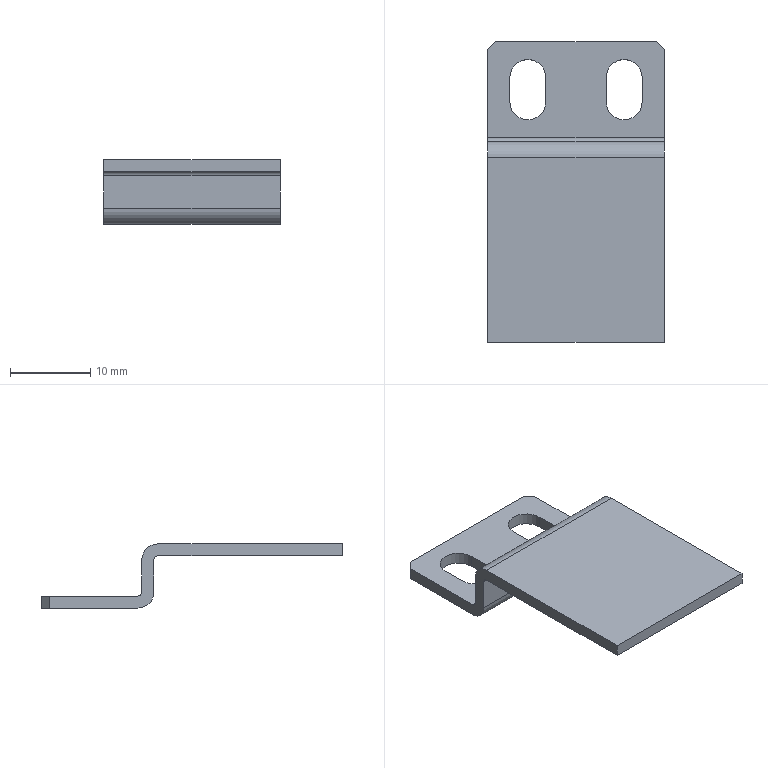Part | SolidWorks | features BaseBody 1 | 1 solid | 24 faces | box 22 x 37.5 x 8 mm | volume 1327 mm3 | plane 16 | cylinder 8 | commonest cylinder face diameters 4.5 x4 1 x2 4 x2
STEP:
#1=CARTESIAN_POINT('',(0.,-37.5,6.5));
#2=VERTEX_POINT('',#1);
#3=CARTESIAN_POINT('',(0.,-14.5,6.5));
#4=VERTEX_POINT('',#3);
#5=CARTESIAN_POINT('',(0.,0.,6.5));
#6=DIRECTION('',(0.,1.,0.));
#7=VECTOR('',#6,1000.);
#8=LINE('',#5,#7);
#9=EDGE_CURVE('',#2,#4,#8,.T.);
#10=ORIENTED_EDGE('',*,*,#9,.F.);
#11=CARTESIAN_POINT('',(22.,-37.5,6.5));
#12=VERTEX_POINT('',#11);
#13=CARTESIAN_POINT('',(0.,-37.5,6.5));
#14=DIRECTION('',(-1.,0.,0.));
#15=VECTOR('',#14,1000.);
#16=LINE('',#13,#15);
#17=EDGE_CURVE('',#12,#2,#16,.T.);
#18=ORIENTED_EDGE('',*,*,#17,.F.);
#19=CARTESIAN_POINT('',(22.,-14.5,6.5));
#20=VERTEX_POINT('',#19);
#21=CARTESIAN_POINT('',(22.,0.,6.5));
#22=DIRECTION('',(0.,-1.,0.));
#23=VECTOR('',#22,1000.);
#24=LINE('',#21,#23);
#25=EDGE_CURVE('',#20,#12,#24,.T.);
#26=ORIENTED_EDGE('',*,*,#25,.F.);
#27=CARTESIAN_POINT('',(0.,-14.5,6.5));
#28=DIRECTION('',(1.,0.,0.));
#29=VECTOR('',#28,1000.);
#30=LINE('',#27,#29);
#31=EDGE_CURVE('',#4,#20,#30,.T.);
#32=ORIENTED_EDGE('',*,*,#31,.F.);
#33=EDGE_LOOP('',(#10,#18,#26,#32));
#34=FACE_OUTER_BOUND('',#33,.T.);
#35=CARTESIAN_POINT('',(0.,0.,6.5));
#36=DIRECTION('',(0.,0.,-1.));
#37=DIRECTION('',(0.,1.,0.));
#38=AXIS2_PLACEMENT_3D('',#35,#36,#37);
#39=PLANE('',#38);
#40=ADVANCED_FACE('',(#34),#39,.F.);
#41=ORIENTED_EDGE('',*,*,#31,.T.);
#42=CARTESIAN_POINT('',(22.,-12.5,4.5));
#43=VERTEX_POINT('',#42);
#44=CARTESIAN_POINT('',(22.,-14.5,4.5));
#45=DIRECTION('',(-1.,0.,0.));
#46=DIRECTION('',(0.,0.,1.));
#47=AXIS2_PLACEMENT_3D('',#44,#45,#46);
#48=CIRCLE('',#47,2.);
#49=EDGE_CURVE('',#20,#43,#48,.T.);
#50=ORIENTED_EDGE('',*,*,#49,.T.);
#51=CARTESIAN_POINT('',(0.,-12.5,4.5));
#52=VERTEX_POINT('',#51);
#53=CARTESIAN_POINT('',(0.,-12.5,4.5));
#54=DIRECTION('',(-1.,0.,0.));
#55=VECTOR('',#54,1000.);
#56=LINE('',#53,#55);
#57=EDGE_CURVE('',#43,#52,#56,.T.);
#58=ORIENTED_EDGE('',*,*,#57,.T.);
#59=CARTESIAN_POINT('',(0.,-14.5,4.5));
#60=DIRECTION('',(1.,0.,0.));
#61=DIRECTION('',(0.,0.,1.));
#62=AXIS2_PLACEMENT_3D('',#59,#60,#61);
#63=CIRCLE('',#62,2.);
#64=EDGE_CURVE('',#52,#4,#63,.T.);
#65=ORIENTED_EDGE('',*,*,#64,.T.);
#66=EDGE_LOOP('',(#41,#50,#58,#65));
#67=FACE_OUTER_BOUND('',#66,.T.);
#68=CARTESIAN_POINT('',(0.,-14.5,4.5));
#69=DIRECTION('',(-1.,0.,0.));
#70=DIRECTION('',(0.,0.,1.));
#71=AXIS2_PLACEMENT_3D('',#68,#69,#70);
#72=CYLINDRICAL_SURFACE('',#71,2.);
#73=ADVANCED_FACE('',(#67),#72,.T.);
#74=CARTESIAN_POINT('',(0.,-37.5,5.));
#75=VERTEX_POINT('',#74);
#76=CARTESIAN_POINT('',(0.,-14.5,5.));
#77=VERTEX_POINT('',#76);
#78=CARTESIAN_POINT('',(0.,-37.5,5.));
#79=DIRECTION('',(0.,1.,0.));
#80=VECTOR('',#79,1000.);
#81=LINE('',#78,#80);
#82=EDGE_CURVE('',#75,#77,#81,.T.);
#83=ORIENTED_EDGE('',*,*,#82,.F.);
#84=CARTESIAN_POINT('',(0.,-37.5,6.5));
#85=DIRECTION('',(0.,0.,-1.));
#86=VECTOR('',#85,1000.);
#87=LINE('',#84,#86);
#88=EDGE_CURVE('',#2,#75,#87,.T.);
#89=ORIENTED_EDGE('',*,*,#88,.F.);
#90=ORIENTED_EDGE('',*,*,#9,.T.);
#91=ORIENTED_EDGE('',*,*,#64,.F.);
#92=CARTESIAN_POINT('',(0.,-12.5,0.5));
#93=VERTEX_POINT('',#92);
#94=CARTESIAN_POINT('',(0.,-12.5,0.));
#95=DIRECTION('',(0.,0.,1.));
#96=VECTOR('',#95,1000.);
#97=LINE('',#94,#96);
#98=EDGE_CURVE('',#93,#52,#97,.T.);
#99=ORIENTED_EDGE('',*,*,#98,.F.);
#100=CARTESIAN_POINT('',(0.,-12.,0.));
#101=VERTEX_POINT('',#100);
#102=CARTESIAN_POINT('',(0.,-12.,0.5));
#103=DIRECTION('',(1.,0.,0.));
#104=DIRECTION('',(0.,0.,-1.));
#105=AXIS2_PLACEMENT_3D('',#102,#103,#104);
#106=CIRCLE('',#105,0.5);
#107=EDGE_CURVE('',#93,#101,#106,.T.);
#108=ORIENTED_EDGE('',*,*,#107,.T.);
#109=CARTESIAN_POINT('',(0.,-1.,0.));
#110=VERTEX_POINT('',#109);
#111=CARTESIAN_POINT('',(0.,0.,0.));
#112=DIRECTION('',(0.,-1.,0.));
#113=VECTOR('',#112,1000.);
#114=LINE('',#111,#113);
#115=EDGE_CURVE('',#110,#101,#114,.T.);
#116=ORIENTED_EDGE('',*,*,#115,.F.);
#117=CARTESIAN_POINT('',(0.,-1.,-1.5));
#118=VERTEX_POINT('',#117);
#119=CARTESIAN_POINT('',(0.,-1.,-1.5));
#120=DIRECTION('',(0.,0.,-1.));
#121=VECTOR('',#120,1000.);
#122=LINE('',#119,#121);
#123=EDGE_CURVE('',#110,#118,#122,.T.);
#124=ORIENTED_EDGE('',*,*,#123,.T.);
#125=CARTESIAN_POINT('',(0.,-12.,-1.5));
#126=VERTEX_POINT('',#125);
#127=CARTESIAN_POINT('',(0.,0.,-1.5));
#128=DIRECTION('',(0.,-1.,0.));
#129=VECTOR('',#128,1000.);
#130=LINE('',#127,#129);
#131=EDGE_CURVE('',#118,#126,#130,.T.);
#132=ORIENTED_EDGE('',*,*,#131,.T.);
#133=CARTESIAN_POINT('',(0.,-14.,0.5));
#134=VERTEX_POINT('',#133);
#135=CARTESIAN_POINT('',(0.,-12.,0.5));
#136=DIRECTION('',(1.,0.,0.));
#137=DIRECTION('',(0.,0.,-1.));
#138=AXIS2_PLACEMENT_3D('',#135,#136,#137);
#139=CIRCLE('',#138,2.);
#140=EDGE_CURVE('',#134,#126,#139,.T.);
#141=ORIENTED_EDGE('',*,*,#140,.F.);
#142=CARTESIAN_POINT('',(0.,-14.,4.5));
#143=VERTEX_POINT('',#142);
#144=CARTESIAN_POINT('',(0.,-14.,0.));
#145=DIRECTION('',(0.,0.,-1.));
#146=VECTOR('',#145,1000.);
#147=LINE('',#144,#146);
#148=EDGE_CURVE('',#143,#134,#147,.T.);
#149=ORIENTED_EDGE('',*,*,#148,.F.);
#150=CARTESIAN_POINT('',(0.,-14.5,4.5));
#151=DIRECTION('',(1.,0.,0.));
#152=DIRECTION('',(0.,0.,1.));
#153=AXIS2_PLACEMENT_3D('',#150,#151,#152);
#154=CIRCLE('',#153,0.5);
#155=EDGE_CURVE('',#143,#77,#154,.T.);
#156=ORIENTED_EDGE('',*,*,#155,.T.);
#157=EDGE_LOOP('',(#83,#89,#90,#91,#99,#108,#116,#124,#132,#141,#149,#156));
#158=FACE_OUTER_BOUND('',#157,.T.);
#159=CARTESIAN_POINT('',(0.,-37.5,6.5));
#160=DIRECTION('',(1.,0.,0.));
#161=DIRECTION('',(0.,0.,-1.));
#162=AXIS2_PLACEMENT_3D('',#159,#160,#161);
#163=PLANE('',#162);
#164=ADVANCED_FACE('',(#158),#163,.F.);
#165=CARTESIAN_POINT('',(22.,-37.5,5.));
#166=VERTEX_POINT('',#165);
#167=CARTESIAN_POINT('',(22.,-37.5,6.5));
#168=DIRECTION('',(0.,0.,-1.));
#169=VECTOR('',#168,1000.);
#170=LINE('',#167,#169);
#171=EDGE_CURVE('',#12,#166,#170,.T.);
#172=ORIENTED_EDGE('',*,*,#171,.F.);
#173=ORIENTED_EDGE('',*,*,#17,.T.);
#174=ORIENTED_EDGE('',*,*,#88,.T.);
#175=CARTESIAN_POINT('',(22.,-37.5,5.));
#176=DIRECTION('',(-1.,0.,0.));
#177=VECTOR('',#176,1000.);
#178=LINE('',#175,#177);
#179=EDGE_CURVE('',#166,#75,#178,.T.);
#180=ORIENTED_EDGE('',*,*,#179,.F.);
#181=EDGE_LOOP('',(#172,#173,#174,#180));
#182=FACE_OUTER_BOUND('',#181,.T.);
#183=CARTESIAN_POINT('',(22.,-37.5,6.5));
#184=DIRECTION('',(0.,1.,0.));
#185=DIRECTION('',(0.,0.,1.));
#186=AXIS2_PLACEMENT_3D('',#183,#184,#185);
#187=PLANE('',#186);
#188=ADVANCED_FACE('',(#182),#187,.F.);
#189=ORIENTED_EDGE('',*,*,#25,.T.);
#190=ORIENTED_EDGE('',*,*,#171,.T.);
#191=CARTESIAN_POINT('',(22.,-14.5,5.));
#192=VERTEX_POINT('',#191);
#193=CARTESIAN_POINT('',(22.,-14.,5.));
#194=DIRECTION('',(0.,-1.,0.));
#195=VECTOR('',#194,1000.);
#196=LINE('',#193,#195);
#197=EDGE_CURVE('',#192,#166,#196,.T.);
#198=ORIENTED_EDGE('',*,*,#197,.F.);
#199=CARTESIAN_POINT('',(22.,-14.,4.5));
#200=VERTEX_POINT('',#199);
#201=CARTESIAN_POINT('',(22.,-14.5,4.5));
#202=DIRECTION('',(-1.,0.,0.));
#203=DIRECTION('',(0.,0.,1.));
#204=AXIS2_PLACEMENT_3D('',#201,#202,#203);
#205=CIRCLE('',#204,0.5);
#206=EDGE_CURVE('',#192,#200,#205,.T.);
#207=ORIENTED_EDGE('',*,*,#206,.T.);
#208=CARTESIAN_POINT('',(22.,-14.,0.5));
#209=VERTEX_POINT('',#208);
#210=CARTESIAN_POINT('',(22.,-14.,4.5));
#211=DIRECTION('',(0.,0.,1.));
#212=VECTOR('',#211,1000.);
#213=LINE('',#210,#212);
#214=EDGE_CURVE('',#209,#200,#213,.T.);
#215=ORIENTED_EDGE('',*,*,#214,.F.);
#216=CARTESIAN_POINT('',(22.,-12.,-1.5));
#217=VERTEX_POINT('',#216);
#218=CARTESIAN_POINT('',(22.,-12.,0.5));
#219=DIRECTION('',(-1.,0.,0.));
#220=DIRECTION('',(0.,0.,-1.));
#221=AXIS2_PLACEMENT_3D('',#218,#219,#220);
#222=CIRCLE('',#221,2.);
#223=EDGE_CURVE('',#217,#209,#222,.T.);
#224=ORIENTED_EDGE('',*,*,#223,.F.);
#225=CARTESIAN_POINT('',(22.,-1.,-1.5));
#226=VERTEX_POINT('',#225);
#227=CARTESIAN_POINT('',(22.,0.,-1.5));
#228=DIRECTION('',(0.,1.,0.));
#229=VECTOR('',#228,1000.);
#230=LINE('',#227,#229);
#231=EDGE_CURVE('',#217,#226,#230,.T.);
#232=ORIENTED_EDGE('',*,*,#231,.T.);
#233=CARTESIAN_POINT('',(22.,-1.,0.));
#234=VERTEX_POINT('',#233);
#235=CARTESIAN_POINT('',(22.,-1.,-1.5));
#236=DIRECTION('',(0.,0.,1.));
#237=VECTOR('',#236,1000.);
#238=LINE('',#235,#237);
#239=EDGE_CURVE('',#226,#234,#238,.T.);
#240=ORIENTED_EDGE('',*,*,#239,.T.);
#241=CARTESIAN_POINT('',(22.,-12.,0.));
#242=VERTEX_POINT('',#241);
#243=CARTESIAN_POINT('',(22.,0.,0.));
#244=DIRECTION('',(0.,1.,0.));
#245=VECTOR('',#244,1000.);
#246=LINE('',#243,#245);
#247=EDGE_CURVE('',#242,#234,#246,.T.);
#248=ORIENTED_EDGE('',*,*,#247,.F.);
#249=CARTESIAN_POINT('',(22.,-12.5,0.5));
#250=VERTEX_POINT('',#249);
#251=CARTESIAN_POINT('',(22.,-12.,0.5));
#252=DIRECTION('',(1.,0.,0.));
#253=DIRECTION('',(0.,0.,-1.));
#254=AXIS2_PLACEMENT_3D('',#251,#252,#253);
#255=CIRCLE('',#254,0.5);
#256=EDGE_CURVE('',#250,#242,#255,.T.);
#257=ORIENTED_EDGE('',*,*,#256,.F.);
#258=CARTESIAN_POINT('',(22.,-12.5,0.));
#259=DIRECTION('',(0.,0.,-1.));
#260=VECTOR('',#259,1000.);
#261=LINE('',#258,#260);
#262=EDGE_CURVE('',#43,#250,#261,.T.);
#263=ORIENTED_EDGE('',*,*,#262,.F.);
#264=ORIENTED_EDGE('',*,*,#49,.F.);
#265=EDGE_LOOP('',(#189,#190,#198,#207,#215,#224,#232,#240,#248,#257,#263,#264));
#266=FACE_OUTER_BOUND('',#265,.T.);
#267=CARTESIAN_POINT('',(22.,-14.,6.5));
#268=DIRECTION('',(-1.,0.,0.));
#269=DIRECTION('',(0.,0.,1.));
#270=AXIS2_PLACEMENT_3D('',#267,#268,#269);
#271=PLANE('',#270);
#272=ADVANCED_FACE('',(#266),#271,.F.);
#273=ORIENTED_EDGE('',*,*,#98,.T.);
#274=ORIENTED_EDGE('',*,*,#57,.F.);
#275=ORIENTED_EDGE('',*,*,#262,.T.);
#276=CARTESIAN_POINT('',(0.,-12.5,0.5));
#277=DIRECTION('',(-1.,0.,0.));
#278=VECTOR('',#277,1000.);
#279=LINE('',#276,#278);
#280=EDGE_CURVE('',#250,#93,#279,.T.);
#281=ORIENTED_EDGE('',*,*,#280,.T.);
#282=EDGE_LOOP('',(#273,#274,#275,#281));
#283=FACE_OUTER_BOUND('',#282,.T.);
#284=CARTESIAN_POINT('',(0.,-12.5,0.));
#285=DIRECTION('',(0.,1.,0.));
#286=DIRECTION('',(0.,0.,1.));
#287=AXIS2_PLACEMENT_3D('',#284,#285,#286);
#288=PLANE('',#287);
#289=ADVANCED_FACE('',(#283),#288,.T.);
#290=ORIENTED_EDGE('',*,*,#197,.T.);
#291=ORIENTED_EDGE('',*,*,#179,.T.);
#292=ORIENTED_EDGE('',*,*,#82,.T.);
#293=CARTESIAN_POINT('',(0.,-14.5,5.));
#294=DIRECTION('',(1.,0.,0.));
#295=VECTOR('',#294,1000.);
#296=LINE('',#293,#295);
#297=EDGE_CURVE('',#77,#192,#296,.T.);
#298=ORIENTED_EDGE('',*,*,#297,.T.);
#299=EDGE_LOOP('',(#290,#291,#292,#298));
#300=FACE_OUTER_BOUND('',#299,.T.);
#301=CARTESIAN_POINT('',(0.,0.,5.));
#302=DIRECTION('',(0.,0.,-1.));
#303=DIRECTION('',(0.,1.,0.));
#304=AXIS2_PLACEMENT_3D('',#301,#302,#303);
#305=PLANE('',#304);
#306=ADVANCED_FACE('',(#300),#305,.T.);
#307=ORIENTED_EDGE('',*,*,#107,.F.);
#308=ORIENTED_EDGE('',*,*,#280,.F.);
#309=ORIENTED_EDGE('',*,*,#256,.T.);
#310=CARTESIAN_POINT('',(22.,-12.,0.));
#311=DIRECTION('',(1.,0.,0.));
#312=VECTOR('',#311,1000.);
#313=LINE('',#310,#312);
#314=EDGE_CURVE('',#101,#242,#313,.T.);
#315=ORIENTED_EDGE('',*,*,#314,.F.);
#316=EDGE_LOOP('',(#307,#308,#309,#315));
#317=FACE_OUTER_BOUND('',#316,.T.);
#318=CARTESIAN_POINT('',(22.,-12.,0.5));
#319=DIRECTION('',(1.,0.,0.));
#320=DIRECTION('',(0.,0.,-1.));
#321=AXIS2_PLACEMENT_3D('',#318,#319,#320);
#322=CYLINDRICAL_SURFACE('',#321,0.5);
#323=ADVANCED_FACE('',(#317),#322,.F.);
#324=ORIENTED_EDGE('',*,*,#206,.F.);
#325=ORIENTED_EDGE('',*,*,#297,.F.);
#326=ORIENTED_EDGE('',*,*,#155,.F.);
#327=CARTESIAN_POINT('',(0.,-14.,4.5));
#328=DIRECTION('',(-1.,0.,0.));
#329=VECTOR('',#328,1000.);
#330=LINE('',#327,#329);
#331=EDGE_CURVE('',#200,#143,#330,.T.);
#332=ORIENTED_EDGE('',*,*,#331,.F.);
#333=EDGE_LOOP('',(#324,#325,#326,#332));
#334=FACE_OUTER_BOUND('',#333,.T.);
#335=CARTESIAN_POINT('',(0.,-14.5,4.5));
#336=DIRECTION('',(-1.,0.,0.));
#337=DIRECTION('',(0.,0.,1.));
#338=AXIS2_PLACEMENT_3D('',#335,#336,#337);
#339=CYLINDRICAL_SURFACE('',#338,0.5);
#340=ADVANCED_FACE('',(#334),#339,.F.);
#341=ORIENTED_EDGE('',*,*,#214,.T.);
#342=ORIENTED_EDGE('',*,*,#331,.T.);
#343=ORIENTED_EDGE('',*,*,#148,.T.);
#344=CARTESIAN_POINT('',(0.,-14.,0.5));
#345=DIRECTION('',(-1.,0.,0.));
#346=VECTOR('',#345,1000.);
#347=LINE('',#344,#346);
#348=EDGE_CURVE('',#209,#134,#347,.T.);
#349=ORIENTED_EDGE('',*,*,#348,.F.);
#350=EDGE_LOOP('',(#341,#342,#343,#349));
#351=FACE_OUTER_BOUND('',#350,.T.);
#352=CARTESIAN_POINT('',(0.,-14.,0.));
#353=DIRECTION('',(0.,1.,0.));
#354=DIRECTION('',(0.,0.,1.));
#355=AXIS2_PLACEMENT_3D('',#352,#353,#354);
#356=PLANE('',#355);
#357=ADVANCED_FACE('',(#351),#356,.F.);
#358=ORIENTED_EDGE('',*,*,#115,.T.);
#359=ORIENTED_EDGE('',*,*,#314,.T.);
#360=ORIENTED_EDGE('',*,*,#247,.T.);
#361=CARTESIAN_POINT('',(21.,0.,0.));
#362=VERTEX_POINT('',#361);
#363=CARTESIAN_POINT('',(22.,-1.,0.));
#364=DIRECTION('',(-0.7071,0.7071,0.));
#365=VECTOR('',#364,1000.);
#366=LINE('',#363,#365);
#367=EDGE_CURVE('',#234,#362,#366,.T.);
#368=ORIENTED_EDGE('',*,*,#367,.T.);
#369=CARTESIAN_POINT('',(1.,0.,0.));
#370=VERTEX_POINT('',#369);
#371=CARTESIAN_POINT('',(0.,0.,0.));
#372=DIRECTION('',(-1.,0.,0.));
#373=VECTOR('',#372,1000.);
#374=LINE('',#371,#373);
#375=EDGE_CURVE('',#362,#370,#374,.T.);
#376=ORIENTED_EDGE('',*,*,#375,.T.);
#377=CARTESIAN_POINT('',(1.,0.,0.));
#378=DIRECTION('',(-0.7071,-0.7071,0.));
#379=VECTOR('',#378,1000.);
#380=LINE('',#377,#379);
#381=EDGE_CURVE('',#370,#110,#380,.T.);
#382=ORIENTED_EDGE('',*,*,#381,.T.);
#383=EDGE_LOOP('',(#358,#359,#360,#368,#376,#382));
#384=FACE_OUTER_BOUND('',#383,.T.);
#385=CARTESIAN_POINT('',(7.25,-7.5,0.));
#386=VERTEX_POINT('',#385);
#387=CARTESIAN_POINT('',(2.75,-7.5,0.));
#388=VERTEX_POINT('',#387);
#389=CARTESIAN_POINT('',(5.,-7.5,0.));
#390=DIRECTION('',(0.,0.,-1.));
#391=DIRECTION('',(1.,0.,0.));
#392=AXIS2_PLACEMENT_3D('',#389,#390,#391);
#393=CIRCLE('',#392,2.25);
#394=EDGE_CURVE('',#386,#388,#393,.T.);
#395=ORIENTED_EDGE('',*,*,#394,.T.);
#396=CARTESIAN_POINT('',(2.75,-4.5,0.));
#397=VERTEX_POINT('',#396);
#398=CARTESIAN_POINT('',(2.75,0.,0.));
#399=DIRECTION('',(0.,1.,0.));
#400=VECTOR('',#399,1000.);
#401=LINE('',#398,#400);
#402=EDGE_CURVE('',#388,#397,#401,.T.);
#403=ORIENTED_EDGE('',*,*,#402,.T.);
#404=CARTESIAN_POINT('',(7.25,-4.5,0.));
#405=VERTEX_POINT('',#404);
#406=CARTESIAN_POINT('',(5.,-4.5,0.));
#407=DIRECTION('',(0.,0.,-1.));
#408=DIRECTION('',(1.,0.,0.));
#409=AXIS2_PLACEMENT_3D('',#406,#407,#408);
#410=CIRCLE('',#409,2.25);
#411=EDGE_CURVE('',#397,#405,#410,.T.);
#412=ORIENTED_EDGE('',*,*,#411,.T.);
#413=CARTESIAN_POINT('',(7.25,0.,0.));
#414=DIRECTION('',(0.,-1.,0.));
#415=VECTOR('',#414,1000.);
#416=LINE('',#413,#415);
#417=EDGE_CURVE('',#405,#386,#416,.T.);
#418=ORIENTED_EDGE('',*,*,#417,.T.);
#419=EDGE_LOOP('',(#395,#403,#412,#418));
#420=FACE_BOUND('',#419,.T.);
#421=CARTESIAN_POINT('',(19.25,-7.5,0.));
#422=VERTEX_POINT('',#421);
#423=CARTESIAN_POINT('',(14.75,-7.5,0.));
#424=VERTEX_POINT('',#423);
#425=CARTESIAN_POINT('',(17.,-7.5,0.));
#426=DIRECTION('',(0.,0.,-1.));
#427=DIRECTION('',(1.,0.,0.));
#428=AXIS2_PLACEMENT_3D('',#425,#426,#427);
#429=CIRCLE('',#428,2.25);
#430=EDGE_CURVE('',#422,#424,#429,.T.);
#431=ORIENTED_EDGE('',*,*,#430,.T.);
#432=CARTESIAN_POINT('',(14.75,-4.5,0.));
#433=VERTEX_POINT('',#432);
#434=CARTESIAN_POINT('',(14.75,0.,0.));
#435=DIRECTION('',(0.,1.,0.));
#436=VECTOR('',#435,1000.);
#437=LINE('',#434,#436);
#438=EDGE_CURVE('',#424,#433,#437,.T.);
#439=ORIENTED_EDGE('',*,*,#438,.T.);
#440=CARTESIAN_POINT('',(19.25,-4.5,0.));
#441=VERTEX_POINT('',#440);
#442=CARTESIAN_POINT('',(17.,-4.5,0.));
#443=DIRECTION('',(0.,0.,-1.));
#444=DIRECTION('',(1.,0.,0.));
#445=AXIS2_PLACEMENT_3D('',#442,#443,#444);
#446=CIRCLE('',#445,2.25);
#447=EDGE_CURVE('',#433,#441,#446,.T.);
#448=ORIENTED_EDGE('',*,*,#447,.T.);
#449=CARTESIAN_POINT('',(19.25,0.,0.));
#450=DIRECTION('',(0.,-1.,0.));
#451=VECTOR('',#450,1000.);
#452=LINE('',#449,#451);
#453=EDGE_CURVE('',#441,#422,#452,.T.);
#454=ORIENTED_EDGE('',*,*,#453,.T.);
#455=EDGE_LOOP('',(#431,#439,#448,#454));
#456=FACE_BOUND('',#455,.T.);
#457=CARTESIAN_POINT('',(0.,0.,0.));
#458=DIRECTION('',(0.,0.,1.));
#459=DIRECTION('',(1.,0.,0.));
#460=AXIS2_PLACEMENT_3D('',#457,#458,#459);
#461=PLANE('',#460);
#462=ADVANCED_FACE('',(#384,#420,#456),#461,.T.);
#463=ORIENTED_EDGE('',*,*,#348,.T.);
#464=ORIENTED_EDGE('',*,*,#140,.T.);
#465=CARTESIAN_POINT('',(22.,-12.,-1.5));
#466=DIRECTION('',(1.,0.,0.));
#467=VECTOR('',#466,1000.);
#468=LINE('',#465,#467);
#469=EDGE_CURVE('',#126,#217,#468,.T.);
#470=ORIENTED_EDGE('',*,*,#469,.T.);
#471=ORIENTED_EDGE('',*,*,#223,.T.);
#472=EDGE_LOOP('',(#463,#464,#470,#471));
#473=FACE_OUTER_BOUND('',#472,.T.);
#474=CARTESIAN_POINT('',(22.,-12.,0.5));
#475=DIRECTION('',(1.,0.,0.));
#476=DIRECTION('',(0.,0.,-1.));
#477=AXIS2_PLACEMENT_3D('',#474,#475,#476);
#478=CYLINDRICAL_SURFACE('',#477,2.);
#479=ADVANCED_FACE('',(#473),#478,.T.);
#480=ORIENTED_EDGE('',*,*,#123,.F.);
#481=ORIENTED_EDGE('',*,*,#381,.F.);
#482=CARTESIAN_POINT('',(1.,0.,-1.5));
#483=VERTEX_POINT('',#482);
#484=CARTESIAN_POINT('',(1.,0.,-1.5));
#485=DIRECTION('',(0.,0.,1.));
#486=VECTOR('',#485,1000.);
#487=LINE('',#484,#486);
#488=EDGE_CURVE('',#483,#370,#487,.T.);
#489=ORIENTED_EDGE('',*,*,#488,.F.);
#490=CARTESIAN_POINT('',(1.,0.,-1.5));
#491=DIRECTION('',(0.7071,0.7071,0.));
#492=VECTOR('',#491,1000.);
#493=LINE('',#490,#492);
#494=EDGE_CURVE('',#118,#483,#493,.T.);
#495=ORIENTED_EDGE('',*,*,#494,.F.);
#496=EDGE_LOOP('',(#480,#481,#489,#495));
#497=FACE_OUTER_BOUND('',#496,.T.);
#498=CARTESIAN_POINT('',(1.,0.,-1.5));
#499=DIRECTION('',(0.7071,-0.7071,0.));
#500=DIRECTION('',(0.7071,0.7071,0.));
#501=AXIS2_PLACEMENT_3D('',#498,#499,#500);
#502=PLANE('',#501);
#503=ADVANCED_FACE('',(#497),#502,.F.);
#504=CARTESIAN_POINT('',(21.,0.,-1.5));
#505=VERTEX_POINT('',#504);
#506=CARTESIAN_POINT('',(0.,0.,-1.5));
#507=DIRECTION('',(-1.,0.,0.));
#508=VECTOR('',#507,1000.);
#509=LINE('',#506,#508);
#510=EDGE_CURVE('',#505,#483,#509,.T.);
#511=ORIENTED_EDGE('',*,*,#510,.T.);
#512=ORIENTED_EDGE('',*,*,#488,.T.);
#513=ORIENTED_EDGE('',*,*,#375,.F.);
#514=CARTESIAN_POINT('',(21.,0.,-1.5));
#515=DIRECTION('',(0.,0.,-1.));
#516=VECTOR('',#515,1000.);
#517=LINE('',#514,#516);
#518=EDGE_CURVE('',#362,#505,#517,.T.);
#519=ORIENTED_EDGE('',*,*,#518,.T.);
#520=EDGE_LOOP('',(#511,#512,#513,#519));
#521=FACE_OUTER_BOUND('',#520,.T.);
#522=CARTESIAN_POINT('',(0.,0.,-1.5));
#523=DIRECTION('',(0.,1.,0.));
#524=DIRECTION('',(0.,0.,1.));
#525=AXIS2_PLACEMENT_3D('',#522,#523,#524);
#526=PLANE('',#525);
#527=ADVANCED_FACE('',(#521),#526,.T.);
#528=ORIENTED_EDGE('',*,*,#518,.F.);
#529=ORIENTED_EDGE('',*,*,#367,.F.);
#530=ORIENTED_EDGE('',*,*,#239,.F.);
#531=CARTESIAN_POINT('',(22.,-1.,-1.5));
#532=DIRECTION('',(0.7071,-0.7071,0.));
#533=VECTOR('',#532,1000.);
#534=LINE('',#531,#533);
#535=EDGE_CURVE('',#505,#226,#534,.T.);
#536=ORIENTED_EDGE('',*,*,#535,.F.);
#537=EDGE_LOOP('',(#528,#529,#530,#536));
#538=FACE_OUTER_BOUND('',#537,.T.);
#539=CARTESIAN_POINT('',(22.,-1.,-1.5));
#540=DIRECTION('',(-0.7071,-0.7071,0.));
#541=DIRECTION('',(0.7071,-0.7071,0.));
#542=AXIS2_PLACEMENT_3D('',#539,#540,#541);
#543=PLANE('',#542);
#544=ADVANCED_FACE('',(#538),#543,.F.);
#545=CARTESIAN_POINT('',(2.75,-7.5,-1.5));
#546=VERTEX_POINT('',#545);
#547=CARTESIAN_POINT('',(2.75,-7.5,-1.5));
#548=DIRECTION('',(0.,0.,1.));
#549=VECTOR('',#548,1000.);
#550=LINE('',#547,#549);
#551=EDGE_CURVE('',#546,#388,#550,.T.);
#552=ORIENTED_EDGE('',*,*,#551,.F.);
#553=CARTESIAN_POINT('',(2.75,-4.5,-1.5));
#554=VERTEX_POINT('',#553);
#555=CARTESIAN_POINT('',(2.75,-4.5,-1.5));
#556=DIRECTION('',(0.,-1.,0.));
#557=VECTOR('',#556,1000.);
#558=LINE('',#555,#557);
#559=EDGE_CURVE('',#554,#546,#558,.T.);
#560=ORIENTED_EDGE('',*,*,#559,.F.);
#561=CARTESIAN_POINT('',(2.75,-4.5,-1.5));
#562=DIRECTION('',(0.,0.,-1.));
#563=VECTOR('',#562,1000.);
#564=LINE('',#561,#563);
#565=EDGE_CURVE('',#397,#554,#564,.T.);
#566=ORIENTED_EDGE('',*,*,#565,.F.);
#567=ORIENTED_EDGE('',*,*,#402,.F.);
#568=EDGE_LOOP('',(#552,#560,#566,#567));
#569=FACE_OUTER_BOUND('',#568,.T.);
#570=CARTESIAN_POINT('',(2.75,-4.5,-1.5));
#571=DIRECTION('',(-1.,0.,0.));
#572=DIRECTION('',(0.,0.,1.));
#573=AXIS2_PLACEMENT_3D('',#570,#571,#572);
#574=PLANE('',#573);
#575=ADVANCED_FACE('',(#569),#574,.F.);
#576=CARTESIAN_POINT('',(7.25,-7.5,-1.5));
#577=VERTEX_POINT('',#576);
#578=CARTESIAN_POINT('',(7.25,-7.5,-1.5));
#579=DIRECTION('',(0.,0.,1.));
#580=VECTOR('',#579,1000.);
#581=LINE('',#578,#580);
#582=EDGE_CURVE('',#577,#386,#581,.T.);
#583=ORIENTED_EDGE('',*,*,#582,.F.);
#584=CARTESIAN_POINT('',(5.,-7.5,-1.5));
#585=DIRECTION('',(0.,0.,1.));
#586=DIRECTION('',(1.,0.,0.));
#587=AXIS2_PLACEMENT_3D('',#584,#585,#586);
#588=CIRCLE('',#587,2.25);
#589=EDGE_CURVE('',#546,#577,#588,.T.);
#590=ORIENTED_EDGE('',*,*,#589,.F.);
#591=ORIENTED_EDGE('',*,*,#551,.T.);
#592=ORIENTED_EDGE('',*,*,#394,.F.);
#593=EDGE_LOOP('',(#583,#590,#591,#592));
#594=FACE_OUTER_BOUND('',#593,.T.);
#595=CARTESIAN_POINT('',(5.,-7.5,-1.5));
#596=DIRECTION('',(0.,0.,1.));
#597=DIRECTION('',(1.,0.,0.));
#598=AXIS2_PLACEMENT_3D('',#595,#596,#597);
#599=CYLINDRICAL_SURFACE('',#598,2.25);
#600=ADVANCED_FACE('',(#594),#599,.F.);
#601=CARTESIAN_POINT('',(7.25,-4.5,-1.5));
#602=VERTEX_POINT('',#601);
#603=CARTESIAN_POINT('',(7.25,-4.5,-1.5));
#604=DIRECTION('',(0.,0.,1.));
#605=VECTOR('',#604,1000.);
#606=LINE('',#603,#605);
#607=EDGE_CURVE('',#602,#405,#606,.T.);
#608=ORIENTED_EDGE('',*,*,#607,.F.);
#609=CARTESIAN_POINT('',(7.25,-4.5,-1.5));
#610=DIRECTION('',(0.,1.,0.));
#611=VECTOR('',#610,1000.);
#612=LINE('',#609,#611);
#613=EDGE_CURVE('',#577,#602,#612,.T.);
#614=ORIENTED_EDGE('',*,*,#613,.F.);
#615=ORIENTED_EDGE('',*,*,#582,.T.);
#616=ORIENTED_EDGE('',*,*,#417,.F.);
#617=EDGE_LOOP('',(#608,#614,#615,#616));
#618=FACE_OUTER_BOUND('',#617,.T.);
#619=CARTESIAN_POINT('',(7.25,-4.5,-1.5));
#620=DIRECTION('',(1.,0.,0.));
#621=DIRECTION('',(0.,0.,-1.));
#622=AXIS2_PLACEMENT_3D('',#619,#620,#621);
#623=PLANE('',#622);
#624=ADVANCED_FACE('',(#618),#623,.F.);
#625=ORIENTED_EDGE('',*,*,#565,.T.);
#626=CARTESIAN_POINT('',(5.,-4.5,-1.5));
#627=DIRECTION('',(0.,0.,1.));
#628=DIRECTION('',(1.,0.,0.));
#629=AXIS2_PLACEMENT_3D('',#626,#627,#628);
#630=CIRCLE('',#629,2.25);
#631=EDGE_CURVE('',#602,#554,#630,.T.);
#632=ORIENTED_EDGE('',*,*,#631,.F.);
#633=ORIENTED_EDGE('',*,*,#607,.T.);
#634=ORIENTED_EDGE('',*,*,#411,.F.);
#635=EDGE_LOOP('',(#625,#632,#633,#634));
#636=FACE_OUTER_BOUND('',#635,.T.);
#637=CARTESIAN_POINT('',(5.,-4.5,-1.5));
#638=DIRECTION('',(0.,0.,1.));
#639=DIRECTION('',(1.,0.,0.));
#640=AXIS2_PLACEMENT_3D('',#637,#638,#639);
#641=CYLINDRICAL_SURFACE('',#640,2.25);
#642=ADVANCED_FACE('',(#636),#641,.F.);
#643=CARTESIAN_POINT('',(14.75,-7.5,-1.5));
#644=VERTEX_POINT('',#643);
#645=CARTESIAN_POINT('',(14.75,-7.5,-1.5));
#646=DIRECTION('',(0.,0.,1.));
#647=VECTOR('',#646,1000.);
#648=LINE('',#645,#647);
#649=EDGE_CURVE('',#644,#424,#648,.T.);
#650=ORIENTED_EDGE('',*,*,#649,.F.);
#651=CARTESIAN_POINT('',(14.75,-4.5,-1.5));
#652=VERTEX_POINT('',#651);
#653=CARTESIAN_POINT('',(14.75,-4.5,-1.5));
#654=DIRECTION('',(0.,-1.,0.));
#655=VECTOR('',#654,1000.);
#656=LINE('',#653,#655);
#657=EDGE_CURVE('',#652,#644,#656,.T.);
#658=ORIENTED_EDGE('',*,*,#657,.F.);
#659=CARTESIAN_POINT('',(14.75,-4.5,-1.5));
#660=DIRECTION('',(0.,0.,-1.));
#661=VECTOR('',#660,1000.);
#662=LINE('',#659,#661);
#663=EDGE_CURVE('',#433,#652,#662,.T.);
#664=ORIENTED_EDGE('',*,*,#663,.F.);
#665=ORIENTED_EDGE('',*,*,#438,.F.);
#666=EDGE_LOOP('',(#650,#658,#664,#665));
#667=FACE_OUTER_BOUND('',#666,.T.);
#668=CARTESIAN_POINT('',(14.75,-4.5,-1.5));
#669=DIRECTION('',(-1.,0.,0.));
#670=DIRECTION('',(0.,0.,1.));
#671=AXIS2_PLACEMENT_3D('',#668,#669,#670);
#672=PLANE('',#671);
#673=ADVANCED_FACE('',(#667),#672,.F.);
#674=CARTESIAN_POINT('',(19.25,-7.5,-1.5));
#675=VERTEX_POINT('',#674);
#676=CARTESIAN_POINT('',(19.25,-7.5,-1.5));
#677=DIRECTION('',(0.,0.,1.));
#678=VECTOR('',#677,1000.);
#679=LINE('',#676,#678);
#680=EDGE_CURVE('',#675,#422,#679,.T.);
#681=ORIENTED_EDGE('',*,*,#680,.F.);
#682=CARTESIAN_POINT('',(17.,-7.5,-1.5));
#683=DIRECTION('',(0.,0.,1.));
#684=DIRECTION('',(1.,0.,0.));
#685=AXIS2_PLACEMENT_3D('',#682,#683,#684);
#686=CIRCLE('',#685,2.25);
#687=EDGE_CURVE('',#644,#675,#686,.T.);
#688=ORIENTED_EDGE('',*,*,#687,.F.);
#689=ORIENTED_EDGE('',*,*,#649,.T.);
#690=ORIENTED_EDGE('',*,*,#430,.F.);
#691=EDGE_LOOP('',(#681,#688,#689,#690));
#692=FACE_OUTER_BOUND('',#691,.T.);
#693=CARTESIAN_POINT('',(17.,-7.5,-1.5));
#694=DIRECTION('',(0.,0.,1.));
#695=DIRECTION('',(1.,0.,0.));
#696=AXIS2_PLACEMENT_3D('',#693,#694,#695);
#697=CYLINDRICAL_SURFACE('',#696,2.25);
#698=ADVANCED_FACE('',(#692),#697,.F.);
#699=CARTESIAN_POINT('',(19.25,-4.5,-1.5));
#700=VERTEX_POINT('',#699);
#701=CARTESIAN_POINT('',(19.25,-4.5,-1.5));
#702=DIRECTION('',(0.,0.,1.));
#703=VECTOR('',#702,1000.);
#704=LINE('',#701,#703);
#705=EDGE_CURVE('',#700,#441,#704,.T.);
#706=ORIENTED_EDGE('',*,*,#705,.F.);
#707=CARTESIAN_POINT('',(19.25,-4.5,-1.5));
#708=DIRECTION('',(0.,1.,0.));
#709=VECTOR('',#708,1000.);
#710=LINE('',#707,#709);
#711=EDGE_CURVE('',#675,#700,#710,.T.);
#712=ORIENTED_EDGE('',*,*,#711,.F.);
#713=ORIENTED_EDGE('',*,*,#680,.T.);
#714=ORIENTED_EDGE('',*,*,#453,.F.);
#715=EDGE_LOOP('',(#706,#712,#713,#714));
#716=FACE_OUTER_BOUND('',#715,.T.);
#717=CARTESIAN_POINT('',(19.25,-4.5,-1.5));
#718=DIRECTION('',(1.,0.,0.));
#719=DIRECTION('',(0.,0.,-1.));
#720=AXIS2_PLACEMENT_3D('',#717,#718,#719);
#721=PLANE('',#720);
#722=ADVANCED_FACE('',(#716),#721,.F.);
#723=ORIENTED_EDGE('',*,*,#663,.T.);
#724=CARTESIAN_POINT('',(17.,-4.5,-1.5));
#725=DIRECTION('',(0.,0.,1.));
#726=DIRECTION('',(1.,0.,0.));
#727=AXIS2_PLACEMENT_3D('',#724,#725,#726);
#728=CIRCLE('',#727,2.25);
#729=EDGE_CURVE('',#700,#652,#728,.T.);
#730=ORIENTED_EDGE('',*,*,#729,.F.);
#731=ORIENTED_EDGE('',*,*,#705,.T.);
#732=ORIENTED_EDGE('',*,*,#447,.F.);
#733=EDGE_LOOP('',(#723,#730,#731,#732));
#734=FACE_OUTER_BOUND('',#733,.T.);
#735=CARTESIAN_POINT('',(17.,-4.5,-1.5));
#736=DIRECTION('',(0.,0.,1.));
#737=DIRECTION('',(1.,0.,0.));
#738=AXIS2_PLACEMENT_3D('',#735,#736,#737);
#739=CYLINDRICAL_SURFACE('',#738,2.25);
#740=ADVANCED_FACE('',(#734),#739,.F.);
#741=ORIENTED_EDGE('',*,*,#535,.T.);
#742=ORIENTED_EDGE('',*,*,#231,.F.);
#743=ORIENTED_EDGE('',*,*,#469,.F.);
#744=ORIENTED_EDGE('',*,*,#131,.F.);
#745=ORIENTED_EDGE('',*,*,#494,.T.);
#746=ORIENTED_EDGE('',*,*,#510,.F.);
#747=EDGE_LOOP('',(#741,#742,#743,#744,#745,#746));
#748=FACE_OUTER_BOUND('',#747,.T.);
#749=ORIENTED_EDGE('',*,*,#631,.T.);
#750=ORIENTED_EDGE('',*,*,#559,.T.);
#751=ORIENTED_EDGE('',*,*,#589,.T.);
#752=ORIENTED_EDGE('',*,*,#613,.T.);
#753=EDGE_LOOP('',(#749,#750,#751,#752));
#754=FACE_BOUND('',#753,.T.);
#755=ORIENTED_EDGE('',*,*,#729,.T.);
#756=ORIENTED_EDGE('',*,*,#657,.T.);
#757=ORIENTED_EDGE('',*,*,#687,.T.);
#758=ORIENTED_EDGE('',*,*,#711,.T.);
#759=EDGE_LOOP('',(#755,#756,#757,#758));
#760=FACE_BOUND('',#759,.T.);
#761=CARTESIAN_POINT('',(0.,0.,-1.5));
#762=DIRECTION('',(0.,0.,1.));
#763=DIRECTION('',(1.,0.,0.));
#764=AXIS2_PLACEMENT_3D('',#761,#762,#763);
#765=PLANE('',#764);
#766=ADVANCED_FACE('',(#748,#754,#760),#765,.F.);
#767=CLOSED_SHELL('',(#40,#73,#164,#188,#272,#289,#306,#323,#340,#357,#462,#479,#503,#527,#544,#575,#600,#624,#642,#673,#698,#722,#740,#766));
#768=MANIFOLD_SOLID_BREP('',#767);
#769=CARTESIAN_POINT('',(0.,0.,0.));
#770=DIRECTION('',(0.,0.,1.));
#771=DIRECTION('',(1.,0.,0.));
#772=AXIS2_PLACEMENT_3D('',#769,#770,#771);
#773=(LENGTH_UNIT()NAMED_UNIT(*)SI_UNIT(.MILLI.,.METRE.));
#774=UNCERTAINTY_MEASURE_WITH_UNIT(LENGTH_MEASURE(0.00001),#773,'','');
#775=(NAMED_UNIT(*)PLANE_ANGLE_UNIT()SI_UNIT($,.RADIAN.));
#776=(NAMED_UNIT(*)SI_UNIT($,.STERADIAN.)SOLID_ANGLE_UNIT());
#777=(GEOMETRIC_REPRESENTATION_CONTEXT(3)GLOBAL_UNCERTAINTY_ASSIGNED_CONTEXT((#774))GLOBAL_UNIT_ASSIGNED_CONTEXT((#773,#775,#776))REPRESENTATION_CONTEXT('',''));
#778=ADVANCED_BREP_SHAPE_REPRESENTATION('',(#768,#772),#777);